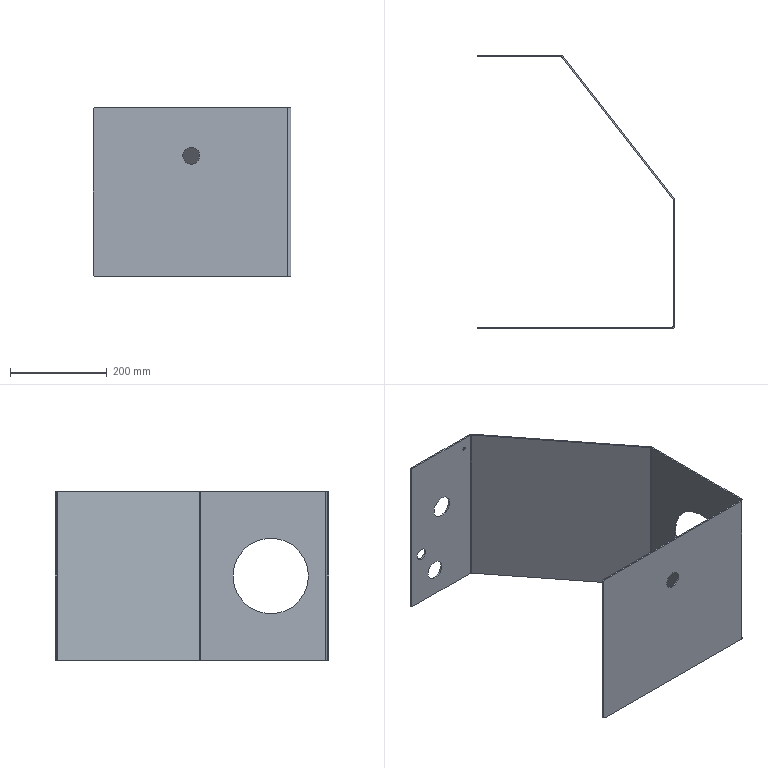Part | SolidWorks | features ICE 4, FlatPattern 1, SMBaseFlange 1, SheetMetal 1 | 1 solid | 46 faces | box 409 x 566 x 350 mm | volume 1214329 mm3 | plane 24 | cylinder 22 | commonest cylinder face diameters 10 x4 6 x3 12 x3 6.1 x2 24.2 x2 35 x2
STEP:
#1=CARTESIAN_POINT('',(152.,563.,321.95));
#2=VERTEX_POINT('',#1);
#3=CARTESIAN_POINT('',(152.,563.,328.05));
#4=VERTEX_POINT('',#3);
#5=CARTESIAN_POINT('',(152.,563.,325.));
#6=DIRECTION('',(0.,1.,0.));
#7=DIRECTION('',(0.,0.,1.));
#8=AXIS2_PLACEMENT_3D('',#5,#6,#7);
#9=CIRCLE('',#8,3.05);
#10=EDGE_CURVE('',#2,#4,#9,.T.);
#11=ORIENTED_EDGE('',*,*,#10,.F.);
#12=CARTESIAN_POINT('',(152.,566.,321.95));
#13=VERTEX_POINT('',#12);
#14=CARTESIAN_POINT('',(152.,556.,321.95));
#15=DIRECTION('',(0.,1.,0.));
#16=VECTOR('',#15,1000.);
#17=LINE('',#14,#16);
#18=EDGE_CURVE('',#2,#13,#17,.T.);
#19=ORIENTED_EDGE('',*,*,#18,.T.);
#20=CARTESIAN_POINT('',(152.,566.,328.05));
#21=VERTEX_POINT('',#20);
#22=CARTESIAN_POINT('',(152.,566.,325.));
#23=DIRECTION('',(0.,1.,0.));
#24=DIRECTION('',(0.,0.,1.));
#25=AXIS2_PLACEMENT_3D('',#22,#23,#24);
#26=CIRCLE('',#25,3.05);
#27=EDGE_CURVE('',#13,#21,#26,.T.);
#28=ORIENTED_EDGE('',*,*,#27,.T.);
#29=CARTESIAN_POINT('',(152.,556.,328.05));
#30=DIRECTION('',(0.,1.,0.));
#31=VECTOR('',#30,1000.);
#32=LINE('',#29,#31);
#33=EDGE_CURVE('',#4,#21,#32,.T.);
#34=ORIENTED_EDGE('',*,*,#33,.F.);
#35=EDGE_LOOP('',(#11,#19,#28,#34));
#36=FACE_OUTER_BOUND('',#35,.T.);
#37=CARTESIAN_POINT('',(152.,556.,325.));
#38=DIRECTION('',(0.,1.,0.));
#39=DIRECTION('',(0.,0.,1.));
#40=AXIS2_PLACEMENT_3D('',#37,#38,#39);
#41=CYLINDRICAL_SURFACE('',#40,3.05);
#42=ADVANCED_FACE('',(#36),#41,.F.);
#43=CARTESIAN_POINT('',(87.,563.,187.4));
#44=VERTEX_POINT('',#43);
#45=CARTESIAN_POINT('',(87.,563.,232.6));
#46=VERTEX_POINT('',#45);
#47=CARTESIAN_POINT('',(87.,563.,210.));
#48=DIRECTION('',(0.,1.,0.));
#49=DIRECTION('',(0.,0.,1.));
#50=AXIS2_PLACEMENT_3D('',#47,#48,#49);
#51=CIRCLE('',#50,22.6);
#52=EDGE_CURVE('',#44,#46,#51,.T.);
#53=ORIENTED_EDGE('',*,*,#52,.F.);
#54=CARTESIAN_POINT('',(87.,566.,187.4));
#55=VERTEX_POINT('',#54);
#56=CARTESIAN_POINT('',(87.,556.,187.4));
#57=DIRECTION('',(0.,1.,0.));
#58=VECTOR('',#57,1000.);
#59=LINE('',#56,#58);
#60=EDGE_CURVE('',#44,#55,#59,.T.);
#61=ORIENTED_EDGE('',*,*,#60,.T.);
#62=CARTESIAN_POINT('',(87.,566.,232.6));
#63=VERTEX_POINT('',#62);
#64=CARTESIAN_POINT('',(87.,566.,210.));
#65=DIRECTION('',(0.,1.,0.));
#66=DIRECTION('',(0.,0.,1.));
#67=AXIS2_PLACEMENT_3D('',#64,#65,#66);
#68=CIRCLE('',#67,22.6);
#69=EDGE_CURVE('',#55,#63,#68,.T.);
#70=ORIENTED_EDGE('',*,*,#69,.T.);
#71=CARTESIAN_POINT('',(87.,556.,232.6));
#72=DIRECTION('',(0.,1.,0.));
#73=VECTOR('',#72,1000.);
#74=LINE('',#71,#73);
#75=EDGE_CURVE('',#46,#63,#74,.T.);
#76=ORIENTED_EDGE('',*,*,#75,.F.);
#77=EDGE_LOOP('',(#53,#61,#70,#76));
#78=FACE_OUTER_BOUND('',#77,.T.);
#79=CARTESIAN_POINT('',(87.,556.,210.));
#80=DIRECTION('',(0.,1.,0.));
#81=DIRECTION('',(0.,0.,1.));
#82=AXIS2_PLACEMENT_3D('',#79,#80,#81);
#83=CYLINDRICAL_SURFACE('',#82,22.6);
#84=ADVANCED_FACE('',(#78),#83,.F.);
#85=CARTESIAN_POINT('',(27.,563.,107.9));
#86=VERTEX_POINT('',#85);
#87=CARTESIAN_POINT('',(27.,563.,132.1));
#88=VERTEX_POINT('',#87);
#89=CARTESIAN_POINT('',(27.,563.,120.));
#90=DIRECTION('',(0.,1.,0.));
#91=DIRECTION('',(0.,0.,1.));
#92=AXIS2_PLACEMENT_3D('',#89,#90,#91);
#93=CIRCLE('',#92,12.1);
#94=EDGE_CURVE('',#86,#88,#93,.T.);
#95=ORIENTED_EDGE('',*,*,#94,.F.);
#96=CARTESIAN_POINT('',(27.,566.,107.9));
#97=VERTEX_POINT('',#96);
#98=CARTESIAN_POINT('',(27.,556.,107.9));
#99=DIRECTION('',(0.,1.,0.));
#100=VECTOR('',#99,1000.);
#101=LINE('',#98,#100);
#102=EDGE_CURVE('',#86,#97,#101,.T.);
#103=ORIENTED_EDGE('',*,*,#102,.T.);
#104=CARTESIAN_POINT('',(27.,566.,132.1));
#105=VERTEX_POINT('',#104);
#106=CARTESIAN_POINT('',(27.,566.,120.));
#107=DIRECTION('',(0.,1.,0.));
#108=DIRECTION('',(0.,0.,1.));
#109=AXIS2_PLACEMENT_3D('',#106,#107,#108);
#110=CIRCLE('',#109,12.1);
#111=EDGE_CURVE('',#97,#105,#110,.T.);
#112=ORIENTED_EDGE('',*,*,#111,.T.);
#113=CARTESIAN_POINT('',(27.,556.,132.1));
#114=DIRECTION('',(0.,1.,0.));
#115=VECTOR('',#114,1000.);
#116=LINE('',#113,#115);
#117=EDGE_CURVE('',#88,#105,#116,.T.);
#118=ORIENTED_EDGE('',*,*,#117,.F.);
#119=EDGE_LOOP('',(#95,#103,#112,#118));
#120=FACE_OUTER_BOUND('',#119,.T.);
#121=CARTESIAN_POINT('',(27.,556.,120.));
#122=DIRECTION('',(0.,1.,0.));
#123=DIRECTION('',(0.,0.,1.));
#124=AXIS2_PLACEMENT_3D('',#121,#122,#123);
#125=CYLINDRICAL_SURFACE('',#124,12.1);
#126=ADVANCED_FACE('',(#120),#125,.F.);
#127=CARTESIAN_POINT('',(67.,563.,40.));
#128=VERTEX_POINT('',#127);
#129=CARTESIAN_POINT('',(67.,563.,80.));
#130=VERTEX_POINT('',#129);
#131=CARTESIAN_POINT('',(67.,563.,60.));
#132=DIRECTION('',(0.,1.,0.));
#133=DIRECTION('',(0.,0.,1.));
#134=AXIS2_PLACEMENT_3D('',#131,#132,#133);
#135=CIRCLE('',#134,20.);
#136=EDGE_CURVE('',#128,#130,#135,.T.);
#137=ORIENTED_EDGE('',*,*,#136,.F.);
#138=CARTESIAN_POINT('',(67.,566.,40.));
#139=VERTEX_POINT('',#138);
#140=CARTESIAN_POINT('',(67.,556.,40.));
#141=DIRECTION('',(0.,1.,0.));
#142=VECTOR('',#141,1000.);
#143=LINE('',#140,#142);
#144=EDGE_CURVE('',#128,#139,#143,.T.);
#145=ORIENTED_EDGE('',*,*,#144,.T.);
#146=CARTESIAN_POINT('',(67.,566.,80.));
#147=VERTEX_POINT('',#146);
#148=CARTESIAN_POINT('',(67.,566.,60.));
#149=DIRECTION('',(0.,1.,0.));
#150=DIRECTION('',(0.,0.,1.));
#151=AXIS2_PLACEMENT_3D('',#148,#149,#150);
#152=CIRCLE('',#151,20.);
#153=EDGE_CURVE('',#139,#147,#152,.T.);
#154=ORIENTED_EDGE('',*,*,#153,.T.);
#155=CARTESIAN_POINT('',(67.,556.,80.));
#156=DIRECTION('',(0.,1.,0.));
#157=VECTOR('',#156,1000.);
#158=LINE('',#155,#157);
#159=EDGE_CURVE('',#130,#147,#158,.T.);
#160=ORIENTED_EDGE('',*,*,#159,.F.);
#161=EDGE_LOOP('',(#137,#145,#154,#160));
#162=FACE_OUTER_BOUND('',#161,.T.);
#163=CARTESIAN_POINT('',(67.,556.,60.));
#164=DIRECTION('',(0.,1.,0.));
#165=DIRECTION('',(0.,0.,1.));
#166=AXIS2_PLACEMENT_3D('',#163,#164,#165);
#167=CYLINDRICAL_SURFACE('',#166,20.);
#168=ADVANCED_FACE('',(#162),#167,.F.);
#169=CARTESIAN_POINT('',(200.,3.,267.5));
#170=VERTEX_POINT('',#169);
#171=CARTESIAN_POINT('',(200.,3.,232.5));
#172=VERTEX_POINT('',#171);
#173=CARTESIAN_POINT('',(200.,3.,250.));
#174=DIRECTION('',(0.,-1.,0.));
#175=DIRECTION('',(0.,0.,-1.));
#176=AXIS2_PLACEMENT_3D('',#173,#174,#175);
#177=CIRCLE('',#176,17.5);
#178=EDGE_CURVE('',#170,#172,#177,.T.);
#179=ORIENTED_EDGE('',*,*,#178,.F.);
#180=CARTESIAN_POINT('',(200.,0.,267.5));
#181=VERTEX_POINT('',#180);
#182=CARTESIAN_POINT('',(200.,10.,267.5));
#183=DIRECTION('',(0.,-1.,0.));
#184=VECTOR('',#183,1000.);
#185=LINE('',#182,#184);
#186=EDGE_CURVE('',#170,#181,#185,.T.);
#187=ORIENTED_EDGE('',*,*,#186,.T.);
#188=CARTESIAN_POINT('',(200.,0.,232.5));
#189=VERTEX_POINT('',#188);
#190=CARTESIAN_POINT('',(200.,0.,250.));
#191=DIRECTION('',(0.,-1.,0.));
#192=DIRECTION('',(0.,0.,-1.));
#193=AXIS2_PLACEMENT_3D('',#190,#191,#192);
#194=CIRCLE('',#193,17.5);
#195=EDGE_CURVE('',#181,#189,#194,.T.);
#196=ORIENTED_EDGE('',*,*,#195,.T.);
#197=CARTESIAN_POINT('',(200.,10.,232.5));
#198=DIRECTION('',(0.,-1.,0.));
#199=VECTOR('',#198,1000.);
#200=LINE('',#197,#199);
#201=EDGE_CURVE('',#172,#189,#200,.T.);
#202=ORIENTED_EDGE('',*,*,#201,.F.);
#203=EDGE_LOOP('',(#179,#187,#196,#202));
#204=FACE_OUTER_BOUND('',#203,.T.);
#205=CARTESIAN_POINT('',(200.,10.,250.));
#206=DIRECTION('',(0.,-1.,0.));
#207=DIRECTION('',(0.,0.,-1.));
#208=AXIS2_PLACEMENT_3D('',#205,#206,#207);
#209=CYLINDRICAL_SURFACE('',#208,17.5);
#210=ADVANCED_FACE('',(#204),#209,.F.);
#211=CARTESIAN_POINT('',(403.,42.,175.));
#212=VERTEX_POINT('',#211);
#213=CARTESIAN_POINT('',(403.,198.,175.));
#214=VERTEX_POINT('',#213);
#215=CARTESIAN_POINT('',(403.,120.,175.));
#216=DIRECTION('',(1.,0.,0.));
#217=DIRECTION('',(0.,1.,0.));
#218=AXIS2_PLACEMENT_3D('',#215,#216,#217);
#219=CIRCLE('',#218,78.);
#220=EDGE_CURVE('',#212,#214,#219,.T.);
#221=ORIENTED_EDGE('',*,*,#220,.F.);
#222=CARTESIAN_POINT('',(406.,42.,175.));
#223=VERTEX_POINT('',#222);
#224=CARTESIAN_POINT('',(396.,42.,175.));
#225=DIRECTION('',(1.,0.,0.));
#226=VECTOR('',#225,1000.);
#227=LINE('',#224,#226);
#228=EDGE_CURVE('',#212,#223,#227,.T.);
#229=ORIENTED_EDGE('',*,*,#228,.T.);
#230=CARTESIAN_POINT('',(406.,198.,175.));
#231=VERTEX_POINT('',#230);
#232=CARTESIAN_POINT('',(406.,120.,175.));
#233=DIRECTION('',(1.,0.,0.));
#234=DIRECTION('',(0.,1.,0.));
#235=AXIS2_PLACEMENT_3D('',#232,#233,#234);
#236=CIRCLE('',#235,78.);
#237=EDGE_CURVE('',#223,#231,#236,.T.);
#238=ORIENTED_EDGE('',*,*,#237,.T.);
#239=CARTESIAN_POINT('',(396.,198.,175.));
#240=DIRECTION('',(1.,0.,0.));
#241=VECTOR('',#240,1000.);
#242=LINE('',#239,#241);
#243=EDGE_CURVE('',#214,#231,#242,.T.);
#244=ORIENTED_EDGE('',*,*,#243,.F.);
#245=EDGE_LOOP('',(#221,#229,#238,#244));
#246=FACE_OUTER_BOUND('',#245,.T.);
#247=CARTESIAN_POINT('',(396.,120.,175.));
#248=DIRECTION('',(1.,0.,0.));
#249=DIRECTION('',(0.,1.,0.));
#250=AXIS2_PLACEMENT_3D('',#247,#248,#249);
#251=CYLINDRICAL_SURFACE('',#250,78.);
#252=ADVANCED_FACE('',(#246),#251,.F.);
#253=CARTESIAN_POINT('',(152.,566.,325.));
#254=DIRECTION('',(0.,1.,0.));
#255=DIRECTION('',(0.,0.,1.));
#256=AXIS2_PLACEMENT_3D('',#253,#254,#255);
#257=CIRCLE('',#256,3.05);
#258=EDGE_CURVE('',#21,#13,#257,.T.);
#259=ORIENTED_EDGE('',*,*,#258,.F.);
#260=ORIENTED_EDGE('',*,*,#27,.F.);
#261=EDGE_LOOP('',(#259,#260));
#262=FACE_BOUND('',#261,.T.);
#263=CARTESIAN_POINT('',(87.,566.,210.));
#264=DIRECTION('',(0.,1.,0.));
#265=DIRECTION('',(0.,0.,1.));
#266=AXIS2_PLACEMENT_3D('',#263,#264,#265);
#267=CIRCLE('',#266,22.6);
#268=EDGE_CURVE('',#63,#55,#267,.T.);
#269=ORIENTED_EDGE('',*,*,#268,.F.);
#270=ORIENTED_EDGE('',*,*,#69,.F.);
#271=EDGE_LOOP('',(#269,#270));
#272=FACE_BOUND('',#271,.T.);
#273=CARTESIAN_POINT('',(27.,566.,120.));
#274=DIRECTION('',(0.,1.,0.));
#275=DIRECTION('',(0.,0.,1.));
#276=AXIS2_PLACEMENT_3D('',#273,#274,#275);
#277=CIRCLE('',#276,12.1);
#278=EDGE_CURVE('',#105,#97,#277,.T.);
#279=ORIENTED_EDGE('',*,*,#278,.F.);
#280=ORIENTED_EDGE('',*,*,#111,.F.);
#281=EDGE_LOOP('',(#279,#280));
#282=FACE_BOUND('',#281,.T.);
#283=CARTESIAN_POINT('',(67.,566.,60.));
#284=DIRECTION('',(0.,1.,0.));
#285=DIRECTION('',(0.,0.,1.));
#286=AXIS2_PLACEMENT_3D('',#283,#284,#285);
#287=CIRCLE('',#286,20.);
#288=EDGE_CURVE('',#147,#139,#287,.T.);
#289=ORIENTED_EDGE('',*,*,#288,.F.);
#290=ORIENTED_EDGE('',*,*,#153,.F.);
#291=EDGE_LOOP('',(#289,#290));
#292=FACE_BOUND('',#291,.T.);
#293=CARTESIAN_POINT('',(2.,566.,0.));
#294=VERTEX_POINT('',#293);
#295=CARTESIAN_POINT('',(170.25,566.,0.));
#296=VERTEX_POINT('',#295);
#297=CARTESIAN_POINT('',(-3.,566.,0.));
#298=DIRECTION('',(1.,0.,0.));
#299=VECTOR('',#298,1000.);
#300=LINE('',#297,#299);
#301=EDGE_CURVE('',#294,#296,#300,.T.);
#302=ORIENTED_EDGE('',*,*,#301,.F.);
#303=CARTESIAN_POINT('',(-3.,566.,5.));
#304=VERTEX_POINT('',#303);
#305=CARTESIAN_POINT('',(2.,566.,5.));
#306=DIRECTION('',(0.,-1.,0.));
#307=DIRECTION('',(0.,0.,1.));
#308=AXIS2_PLACEMENT_3D('',#305,#306,#307);
#309=CIRCLE('',#308,5.);
#310=EDGE_CURVE('',#304,#294,#309,.T.);
#311=ORIENTED_EDGE('',*,*,#310,.F.);
#312=CARTESIAN_POINT('',(-3.,566.,345.));
#313=VERTEX_POINT('',#312);
#314=CARTESIAN_POINT('',(-3.,566.,350.));
#315=DIRECTION('',(0.,0.,-1.));
#316=VECTOR('',#315,1000.);
#317=LINE('',#314,#316);
#318=EDGE_CURVE('',#313,#304,#317,.T.);
#319=ORIENTED_EDGE('',*,*,#318,.F.);
#320=CARTESIAN_POINT('',(2.,566.,350.));
#321=VERTEX_POINT('',#320);
#322=CARTESIAN_POINT('',(2.,566.,345.));
#323=DIRECTION('',(0.,-1.,0.));
#324=DIRECTION('',(0.,0.,1.));
#325=AXIS2_PLACEMENT_3D('',#322,#323,#324);
#326=CIRCLE('',#325,5.);
#327=EDGE_CURVE('',#321,#313,#326,.T.);
#328=ORIENTED_EDGE('',*,*,#327,.F.);
#329=CARTESIAN_POINT('',(170.25,566.,350.));
#330=VERTEX_POINT('',#329);
#331=CARTESIAN_POINT('',(-3.,566.,350.));
#332=DIRECTION('',(1.,0.,0.));
#333=VECTOR('',#332,1000.);
#334=LINE('',#331,#333);
#335=EDGE_CURVE('',#321,#330,#334,.T.);
#336=ORIENTED_EDGE('',*,*,#335,.T.);
#337=CARTESIAN_POINT('',(170.25,566.,350.));
#338=DIRECTION('',(0.,0.,-1.));
#339=VECTOR('',#338,1000.);
#340=LINE('',#337,#339);
#341=EDGE_CURVE('',#330,#296,#340,.T.);
#342=ORIENTED_EDGE('',*,*,#341,.T.);
#343=EDGE_LOOP('',(#302,#311,#319,#328,#336,#342));
#344=FACE_OUTER_BOUND('',#343,.T.);
#345=CARTESIAN_POINT('',(-3.,566.,350.));
#346=DIRECTION('',(0.,1.,0.));
#347=DIRECTION('',(0.,0.,1.));
#348=AXIS2_PLACEMENT_3D('',#345,#346,#347);
#349=PLANE('',#348);
#350=ADVANCED_FACE('',(#262,#272,#282,#292,#344),#349,.T.);
#351=CARTESIAN_POINT('',(152.,563.,325.));
#352=DIRECTION('',(0.,1.,0.));
#353=DIRECTION('',(0.,0.,1.));
#354=AXIS2_PLACEMENT_3D('',#351,#352,#353);
#355=CIRCLE('',#354,3.05);
#356=EDGE_CURVE('',#4,#2,#355,.T.);
#357=ORIENTED_EDGE('',*,*,#356,.T.);
#358=ORIENTED_EDGE('',*,*,#10,.T.);
#359=EDGE_LOOP('',(#357,#358));
#360=FACE_BOUND('',#359,.T.);
#361=CARTESIAN_POINT('',(87.,563.,210.));
#362=DIRECTION('',(0.,1.,0.));
#363=DIRECTION('',(0.,0.,1.));
#364=AXIS2_PLACEMENT_3D('',#361,#362,#363);
#365=CIRCLE('',#364,22.6);
#366=EDGE_CURVE('',#46,#44,#365,.T.);
#367=ORIENTED_EDGE('',*,*,#366,.T.);
#368=ORIENTED_EDGE('',*,*,#52,.T.);
#369=EDGE_LOOP('',(#367,#368));
#370=FACE_BOUND('',#369,.T.);
#371=CARTESIAN_POINT('',(27.,563.,120.));
#372=DIRECTION('',(0.,1.,0.));
#373=DIRECTION('',(0.,0.,1.));
#374=AXIS2_PLACEMENT_3D('',#371,#372,#373);
#375=CIRCLE('',#374,12.1);
#376=EDGE_CURVE('',#88,#86,#375,.T.);
#377=ORIENTED_EDGE('',*,*,#376,.T.);
#378=ORIENTED_EDGE('',*,*,#94,.T.);
#379=EDGE_LOOP('',(#377,#378));
#380=FACE_BOUND('',#379,.T.);
#381=CARTESIAN_POINT('',(67.,563.,60.));
#382=DIRECTION('',(0.,1.,0.));
#383=DIRECTION('',(0.,0.,1.));
#384=AXIS2_PLACEMENT_3D('',#381,#382,#383);
#385=CIRCLE('',#384,20.);
#386=EDGE_CURVE('',#130,#128,#385,.T.);
#387=ORIENTED_EDGE('',*,*,#386,.T.);
#388=ORIENTED_EDGE('',*,*,#136,.T.);
#389=EDGE_LOOP('',(#387,#388));
#390=FACE_BOUND('',#389,.T.);
#391=CARTESIAN_POINT('',(-3.,563.,5.));
#392=VERTEX_POINT('',#391);
#393=CARTESIAN_POINT('',(2.,563.,0.));
#394=VERTEX_POINT('',#393);
#395=CARTESIAN_POINT('',(2.,563.,5.));
#396=DIRECTION('',(0.,-1.,0.));
#397=DIRECTION('',(0.,0.,1.));
#398=AXIS2_PLACEMENT_3D('',#395,#396,#397);
#399=CIRCLE('',#398,5.);
#400=EDGE_CURVE('',#392,#394,#399,.T.);
#401=ORIENTED_EDGE('',*,*,#400,.T.);
#402=CARTESIAN_POINT('',(170.25,563.,0.));
#403=VERTEX_POINT('',#402);
#404=CARTESIAN_POINT('',(-3.,563.,0.));
#405=DIRECTION('',(1.,0.,0.));
#406=VECTOR('',#405,1000.);
#407=LINE('',#404,#406);
#408=EDGE_CURVE('',#394,#403,#407,.T.);
#409=ORIENTED_EDGE('',*,*,#408,.T.);
#410=CARTESIAN_POINT('',(170.25,563.,350.));
#411=VERTEX_POINT('',#410);
#412=CARTESIAN_POINT('',(170.25,563.,350.));
#413=DIRECTION('',(0.,0.,-1.));
#414=VECTOR('',#413,1000.);
#415=LINE('',#412,#414);
#416=EDGE_CURVE('',#411,#403,#415,.T.);
#417=ORIENTED_EDGE('',*,*,#416,.F.);
#418=CARTESIAN_POINT('',(2.,563.,350.));
#419=VERTEX_POINT('',#418);
#420=CARTESIAN_POINT('',(-3.,563.,350.));
#421=DIRECTION('',(1.,0.,0.));
#422=VECTOR('',#421,1000.);
#423=LINE('',#420,#422);
#424=EDGE_CURVE('',#419,#411,#423,.T.);
#425=ORIENTED_EDGE('',*,*,#424,.F.);
#426=CARTESIAN_POINT('',(-3.,563.,345.));
#427=VERTEX_POINT('',#426);
#428=CARTESIAN_POINT('',(2.,563.,345.));
#429=DIRECTION('',(0.,-1.,0.));
#430=DIRECTION('',(0.,0.,1.));
#431=AXIS2_PLACEMENT_3D('',#428,#429,#430);
#432=CIRCLE('',#431,5.);
#433=EDGE_CURVE('',#419,#427,#432,.T.);
#434=ORIENTED_EDGE('',*,*,#433,.T.);
#435=CARTESIAN_POINT('',(-3.,563.,350.));
#436=DIRECTION('',(0.,0.,-1.));
#437=VECTOR('',#436,1000.);
#438=LINE('',#435,#437);
#439=EDGE_CURVE('',#427,#392,#438,.T.);
#440=ORIENTED_EDGE('',*,*,#439,.T.);
#441=EDGE_LOOP('',(#401,#409,#417,#425,#434,#440));
#442=FACE_OUTER_BOUND('',#441,.T.);
#443=CARTESIAN_POINT('',(-3.,563.,350.));
#444=DIRECTION('',(0.,1.,0.));
#445=DIRECTION('',(0.,0.,1.));
#446=AXIS2_PLACEMENT_3D('',#443,#444,#445);
#447=PLANE('',#446);
#448=ADVANCED_FACE('',(#360,#370,#380,#390,#442),#447,.F.);
#449=ORIENTED_EDGE('',*,*,#408,.F.);
#450=CARTESIAN_POINT('',(2.,563.,0.));
#451=DIRECTION('',(0.,1.,0.));
#452=VECTOR('',#451,1000.);
#453=LINE('',#450,#452);
#454=EDGE_CURVE('',#394,#294,#453,.T.);
#455=ORIENTED_EDGE('',*,*,#454,.T.);
#456=ORIENTED_EDGE('',*,*,#301,.T.);
#457=CARTESIAN_POINT('',(170.25,566.,0.));
#458=DIRECTION('',(0.,-1.,0.));
#459=VECTOR('',#458,1000.);
#460=LINE('',#457,#459);
#461=EDGE_CURVE('',#296,#403,#460,.T.);
#462=ORIENTED_EDGE('',*,*,#461,.T.);
#463=EDGE_LOOP('',(#449,#455,#456,#462));
#464=FACE_OUTER_BOUND('',#463,.T.);
#465=CARTESIAN_POINT('',(172.615,561.847,0.));
#466=DIRECTION('',(0.,0.,-1.));
#467=DIRECTION('',(-1.,0.,0.));
#468=AXIS2_PLACEMENT_3D('',#465,#466,#467);
#469=PLANE('',#468);
#470=ADVANCED_FACE('',(#464),#469,.T.);
#471=CARTESIAN_POINT('',(200.,0.,250.));
#472=DIRECTION('',(0.,-1.,0.));
#473=DIRECTION('',(0.,0.,-1.));
#474=AXIS2_PLACEMENT_3D('',#471,#472,#473);
#475=CIRCLE('',#474,17.5);
#476=EDGE_CURVE('',#189,#181,#475,.T.);
#477=ORIENTED_EDGE('',*,*,#476,.F.);
#478=ORIENTED_EDGE('',*,*,#195,.F.);
#479=EDGE_LOOP('',(#477,#478));
#480=FACE_BOUND('',#479,.T.);
#481=CARTESIAN_POINT('',(-3.,0.,345.));
#482=VERTEX_POINT('',#481);
#483=CARTESIAN_POINT('',(-3.,0.,5.));
#484=VERTEX_POINT('',#483);
#485=CARTESIAN_POINT('',(-3.,0.,350.));
#486=DIRECTION('',(0.,0.,-1.));
#487=VECTOR('',#486,1000.);
#488=LINE('',#485,#487);
#489=EDGE_CURVE('',#482,#484,#488,.T.);
#490=ORIENTED_EDGE('',*,*,#489,.T.);
#491=CARTESIAN_POINT('',(2.,0.,0.));
#492=VERTEX_POINT('',#491);
#493=CARTESIAN_POINT('',(2.,0.,5.));
#494=DIRECTION('',(0.,1.,0.));
#495=DIRECTION('',(0.,0.,-1.));
#496=AXIS2_PLACEMENT_3D('',#493,#494,#495);
#497=CIRCLE('',#496,5.);
#498=EDGE_CURVE('',#492,#484,#497,.T.);
#499=ORIENTED_EDGE('',*,*,#498,.F.);
#500=CARTESIAN_POINT('',(400.,0.,0.));
#501=VERTEX_POINT('',#500);
#502=CARTESIAN_POINT('',(0.,0.,0.));
#503=DIRECTION('',(-1.,0.,0.));
#504=VECTOR('',#503,1000.);
#505=LINE('',#502,#504);
#506=EDGE_CURVE('',#501,#492,#505,.T.);
#507=ORIENTED_EDGE('',*,*,#506,.F.);
#508=CARTESIAN_POINT('',(400.,0.,350.));
#509=VERTEX_POINT('',#508);
#510=CARTESIAN_POINT('',(400.,0.,350.));
#511=DIRECTION('',(0.,0.,-1.));
#512=VECTOR('',#511,1000.);
#513=LINE('',#510,#512);
#514=EDGE_CURVE('',#509,#501,#513,.T.);
#515=ORIENTED_EDGE('',*,*,#514,.F.);
#516=CARTESIAN_POINT('',(2.,0.,350.));
#517=VERTEX_POINT('',#516);
#518=CARTESIAN_POINT('',(0.,0.,350.));
#519=DIRECTION('',(-1.,0.,0.));
#520=VECTOR('',#519,1000.);
#521=LINE('',#518,#520);
#522=EDGE_CURVE('',#509,#517,#521,.T.);
#523=ORIENTED_EDGE('',*,*,#522,.T.);
#524=CARTESIAN_POINT('',(2.,0.,345.));
#525=DIRECTION('',(0.,1.,0.));
#526=DIRECTION('',(0.,0.,-1.));
#527=AXIS2_PLACEMENT_3D('',#524,#525,#526);
#528=CIRCLE('',#527,5.);
#529=EDGE_CURVE('',#482,#517,#528,.T.);
#530=ORIENTED_EDGE('',*,*,#529,.F.);
#531=EDGE_LOOP('',(#490,#499,#507,#515,#523,#530));
#532=FACE_OUTER_BOUND('',#531,.T.);
#533=CARTESIAN_POINT('',(0.,0.,350.));
#534=DIRECTION('',(0.,-1.,0.));
#535=DIRECTION('',(0.,0.,-1.));
#536=AXIS2_PLACEMENT_3D('',#533,#534,#535);
#537=PLANE('',#536);
#538=ADVANCED_FACE('',(#480,#532),#537,.T.);
#539=CARTESIAN_POINT('',(200.,3.,250.));
#540=DIRECTION('',(0.,-1.,0.));
#541=DIRECTION('',(0.,0.,-1.));
#542=AXIS2_PLACEMENT_3D('',#539,#540,#541);
#543=CIRCLE('',#542,17.5);
#544=EDGE_CURVE('',#172,#170,#543,.T.);
#545=ORIENTED_EDGE('',*,*,#544,.T.);
#546=ORIENTED_EDGE('',*,*,#178,.T.);
#547=EDGE_LOOP('',(#545,#546));
#548=FACE_BOUND('',#547,.T.);
#549=CARTESIAN_POINT('',(2.,3.,0.));
#550=VERTEX_POINT('',#549);
#551=CARTESIAN_POINT('',(-3.,3.,5.));
#552=VERTEX_POINT('',#551);
#553=CARTESIAN_POINT('',(2.,3.,5.));
#554=DIRECTION('',(0.,1.,0.));
#555=DIRECTION('',(0.,0.,-1.));
#556=AXIS2_PLACEMENT_3D('',#553,#554,#555);
#557=CIRCLE('',#556,5.);
#558=EDGE_CURVE('',#550,#552,#557,.T.);
#559=ORIENTED_EDGE('',*,*,#558,.T.);
#560=CARTESIAN_POINT('',(-3.,3.,345.));
#561=VERTEX_POINT('',#560);
#562=CARTESIAN_POINT('',(-3.,3.,350.));
#563=DIRECTION('',(0.,0.,-1.));
#564=VECTOR('',#563,1000.);
#565=LINE('',#562,#564);
#566=EDGE_CURVE('',#561,#552,#565,.T.);
#567=ORIENTED_EDGE('',*,*,#566,.F.);
#568=CARTESIAN_POINT('',(2.,3.,350.));
#569=VERTEX_POINT('',#568);
#570=CARTESIAN_POINT('',(2.,3.,345.));
#571=DIRECTION('',(0.,1.,0.));
#572=DIRECTION('',(0.,0.,-1.));
#573=AXIS2_PLACEMENT_3D('',#570,#571,#572);
#574=CIRCLE('',#573,5.);
#575=EDGE_CURVE('',#561,#569,#574,.T.);
#576=ORIENTED_EDGE('',*,*,#575,.T.);
#577=CARTESIAN_POINT('',(400.,3.,350.));
#578=VERTEX_POINT('',#577);
#579=CARTESIAN_POINT('',(0.,3.,350.));
#580=DIRECTION('',(-1.,0.,0.));
#581=VECTOR('',#580,1000.);
#582=LINE('',#579,#581);
#583=EDGE_CURVE('',#578,#569,#582,.T.);
#584=ORIENTED_EDGE('',*,*,#583,.F.);
#585=CARTESIAN_POINT('',(400.,3.,0.));
#586=VERTEX_POINT('',#585);
#587=CARTESIAN_POINT('',(400.,3.,350.));
#588=DIRECTION('',(0.,0.,-1.));
#589=VECTOR('',#588,1000.);
#590=LINE('',#587,#589);
#591=EDGE_CURVE('',#578,#586,#590,.T.);
#592=ORIENTED_EDGE('',*,*,#591,.T.);
#593=CARTESIAN_POINT('',(0.,3.,0.));
#594=DIRECTION('',(-1.,0.,0.));
#595=VECTOR('',#594,1000.);
#596=LINE('',#593,#595);
#597=EDGE_CURVE('',#586,#550,#596,.T.);
#598=ORIENTED_EDGE('',*,*,#597,.T.);
#599=EDGE_LOOP('',(#559,#567,#576,#584,#592,#598));
#600=FACE_OUTER_BOUND('',#599,.T.);
#601=CARTESIAN_POINT('',(0.,3.,350.));
#602=DIRECTION('',(0.,-1.,0.));
#603=DIRECTION('',(0.,0.,-1.));
#604=AXIS2_PLACEMENT_3D('',#601,#602,#603);
#605=PLANE('',#604);
#606=ADVANCED_FACE('',(#548,#600),#605,.F.);
#607=ORIENTED_EDGE('',*,*,#566,.T.);
#608=CARTESIAN_POINT('',(-3.,3.,5.));
#609=DIRECTION('',(0.,-1.,0.));
#610=VECTOR('',#609,1000.);
#611=LINE('',#608,#610);
#612=EDGE_CURVE('',#552,#484,#611,.T.);
#613=ORIENTED_EDGE('',*,*,#612,.T.);
#614=ORIENTED_EDGE('',*,*,#489,.F.);
#615=CARTESIAN_POINT('',(-3.,3.,345.));
#616=DIRECTION('',(0.,-1.,0.));
#617=VECTOR('',#616,1000.);
#618=LINE('',#615,#617);
#619=EDGE_CURVE('',#561,#482,#618,.T.);
#620=ORIENTED_EDGE('',*,*,#619,.F.);
#621=EDGE_LOOP('',(#607,#613,#614,#620));
#622=FACE_OUTER_BOUND('',#621,.T.);
#623=CARTESIAN_POINT('',(-3.,0.,350.));
#624=DIRECTION('',(-1.,0.,0.));
#625=DIRECTION('',(0.,-1.,0.));
#626=AXIS2_PLACEMENT_3D('',#623,#624,#625);
#627=PLANE('',#626);
#628=ADVANCED_FACE('',(#622),#627,.T.);
#629=CARTESIAN_POINT('',(-3.,563.,5.));
#630=DIRECTION('',(0.,1.,0.));
#631=VECTOR('',#630,1000.);
#632=LINE('',#629,#631);
#633=EDGE_CURVE('',#392,#304,#632,.T.);
#634=ORIENTED_EDGE('',*,*,#633,.F.);
#635=ORIENTED_EDGE('',*,*,#439,.F.);
#636=CARTESIAN_POINT('',(-3.,563.,345.));
#637=DIRECTION('',(0.,1.,0.));
#638=VECTOR('',#637,1000.);
#639=LINE('',#636,#638);
#640=EDGE_CURVE('',#427,#313,#639,.T.);
#641=ORIENTED_EDGE('',*,*,#640,.T.);
#642=ORIENTED_EDGE('',*,*,#318,.T.);
#643=EDGE_LOOP('',(#634,#635,#641,#642));
#644=FACE_OUTER_BOUND('',#643,.T.);
#645=CARTESIAN_POINT('',(-3.,563.,350.));
#646=DIRECTION('',(-1.,0.,0.));
#647=DIRECTION('',(0.,0.,1.));
#648=AXIS2_PLACEMENT_3D('',#645,#646,#647);
#649=PLANE('',#648);
#650=ADVANCED_FACE('',(#644),#649,.T.);
#651=CARTESIAN_POINT('',(2.,563.,350.));
#652=DIRECTION('',(0.,1.,0.));
#653=VECTOR('',#652,1000.);
#654=LINE('',#651,#653);
#655=EDGE_CURVE('',#419,#321,#654,.T.);
#656=ORIENTED_EDGE('',*,*,#655,.F.);
#657=ORIENTED_EDGE('',*,*,#424,.T.);
#658=CARTESIAN_POINT('',(170.25,563.,350.));
#659=DIRECTION('',(0.,1.,0.));
#660=VECTOR('',#659,1000.);
#661=LINE('',#658,#660);
#662=EDGE_CURVE('',#411,#330,#661,.T.);
#663=ORIENTED_EDGE('',*,*,#662,.T.);
#664=ORIENTED_EDGE('',*,*,#335,.F.);
#665=EDGE_LOOP('',(#656,#657,#663,#664));
#666=FACE_OUTER_BOUND('',#665,.T.);
#667=CARTESIAN_POINT('',(400.,6.,350.));
#668=DIRECTION('',(0.,0.,-1.));
#669=DIRECTION('',(-1.,0.,0.));
#670=AXIS2_PLACEMENT_3D('',#667,#668,#669);
#671=PLANE('',#670);
#672=ADVANCED_FACE('',(#666),#671,.F.);
#673=ORIENTED_EDGE('',*,*,#583,.T.);
#674=CARTESIAN_POINT('',(2.,3.,350.));
#675=DIRECTION('',(0.,-1.,0.));
#676=VECTOR('',#675,1000.);
#677=LINE('',#674,#676);
#678=EDGE_CURVE('',#569,#517,#677,.T.);
#679=ORIENTED_EDGE('',*,*,#678,.T.);
#680=ORIENTED_EDGE('',*,*,#522,.F.);
#681=CARTESIAN_POINT('',(400.,0.,350.));
#682=DIRECTION('',(0.,1.,0.));
#683=VECTOR('',#682,1000.);
#684=LINE('',#681,#683);
#685=EDGE_CURVE('',#509,#578,#684,.T.);
#686=ORIENTED_EDGE('',*,*,#685,.T.);
#687=EDGE_LOOP('',(#673,#679,#680,#686));
#688=FACE_OUTER_BOUND('',#687,.T.);
#689=CARTESIAN_POINT('',(403.,6.,350.));
#690=DIRECTION('',(0.,0.,1.));
#691=DIRECTION('',(1.,0.,0.));
#692=AXIS2_PLACEMENT_3D('',#689,#690,#691);
#693=PLANE('',#692);
#694=ADVANCED_FACE('',(#688),#693,.T.);
#695=ORIENTED_EDGE('',*,*,#685,.F.);
#696=CARTESIAN_POINT('',(406.,6.,350.));
#697=VERTEX_POINT('',#696);
#698=CARTESIAN_POINT('',(400.,6.,350.));
#699=DIRECTION('',(0.,0.,-1.));
#700=DIRECTION('',(-1.,0.,0.));
#701=AXIS2_PLACEMENT_3D('',#698,#699,#700);
#702=CIRCLE('',#701,6.);
#703=EDGE_CURVE('',#697,#509,#702,.T.);
#704=ORIENTED_EDGE('',*,*,#703,.F.);
#705=CARTESIAN_POINT('',(403.,6.,350.));
#706=VERTEX_POINT('',#705);
#707=CARTESIAN_POINT('',(403.,6.,350.));
#708=DIRECTION('',(1.,0.,0.));
#709=VECTOR('',#708,1000.);
#710=LINE('',#707,#709);
#711=EDGE_CURVE('',#706,#697,#710,.T.);
#712=ORIENTED_EDGE('',*,*,#711,.F.);
#713=CARTESIAN_POINT('',(400.,6.,350.));
#714=DIRECTION('',(0.,0.,-1.));
#715=DIRECTION('',(1.,0.,0.));
#716=AXIS2_PLACEMENT_3D('',#713,#714,#715);
#717=CIRCLE('',#716,3.);
#718=EDGE_CURVE('',#706,#578,#717,.T.);
#719=ORIENTED_EDGE('',*,*,#718,.T.);
#720=EDGE_LOOP('',(#695,#704,#712,#719));
#721=FACE_OUTER_BOUND('',#720,.T.);
#722=CARTESIAN_POINT('',(400.,0.,350.));
#723=DIRECTION('',(0.,0.,1.));
#724=DIRECTION('',(1.,0.,0.));
#725=AXIS2_PLACEMENT_3D('',#722,#723,#724);
#726=PLANE('',#725);
#727=ADVANCED_FACE('',(#721),#726,.T.);
#728=CARTESIAN_POINT('',(406.,6.,0.));
#729=VERTEX_POINT('',#728);
#730=CARTESIAN_POINT('',(403.,6.,0.));
#731=VERTEX_POINT('',#730);
#732=CARTESIAN_POINT('',(406.,6.,0.));
#733=DIRECTION('',(-1.,0.,0.));
#734=VECTOR('',#733,1000.);
#735=LINE('',#732,#734);
#736=EDGE_CURVE('',#729,#731,#735,.T.);
#737=ORIENTED_EDGE('',*,*,#736,.F.);
#738=CARTESIAN_POINT('',(400.,6.,0.));
#739=DIRECTION('',(0.,0.,-1.));
#740=DIRECTION('',(-1.,0.,0.));
#741=AXIS2_PLACEMENT_3D('',#738,#739,#740);
#742=CIRCLE('',#741,6.);
#743=EDGE_CURVE('',#729,#501,#742,.T.);
#744=ORIENTED_EDGE('',*,*,#743,.T.);
#745=CARTESIAN_POINT('',(400.,3.,0.));
#746=DIRECTION('',(0.,-1.,0.));
#747=VECTOR('',#746,1000.);
#748=LINE('',#745,#747);
#749=EDGE_CURVE('',#586,#501,#748,.T.);
#750=ORIENTED_EDGE('',*,*,#749,.F.);
#751=CARTESIAN_POINT('',(400.,6.,0.));
#752=DIRECTION('',(0.,0.,-1.));
#753=DIRECTION('',(1.,0.,0.));
#754=AXIS2_PLACEMENT_3D('',#751,#752,#753);
#755=CIRCLE('',#754,3.);
#756=EDGE_CURVE('',#731,#586,#755,.T.);
#757=ORIENTED_EDGE('',*,*,#756,.F.);
#758=EDGE_LOOP('',(#737,#744,#750,#757));
#759=FACE_OUTER_BOUND('',#758,.T.);
#760=CARTESIAN_POINT('',(406.,6.,0.));
#761=DIRECTION('',(0.,0.,-1.));
#762=DIRECTION('',(-1.,0.,0.));
#763=AXIS2_PLACEMENT_3D('',#760,#761,#762);
#764=PLANE('',#763);
#765=ADVANCED_FACE('',(#759),#764,.T.);
#766=CARTESIAN_POINT('',(406.,265.934,0.));
#767=VERTEX_POINT('',#766);
#768=CARTESIAN_POINT('',(406.,0.,0.));
#769=DIRECTION('',(0.,-1.,0.));
#770=VECTOR('',#769,1000.);
#771=LINE('',#768,#770);
#772=EDGE_CURVE('',#767,#729,#771,.T.);
#773=ORIENTED_EDGE('',*,*,#772,.T.);
#774=ORIENTED_EDGE('',*,*,#736,.T.);
#775=CARTESIAN_POINT('',(403.,265.934,0.));
#776=VERTEX_POINT('',#775);
#777=CARTESIAN_POINT('',(403.,0.,0.));
#778=DIRECTION('',(0.,-1.,0.));
#779=VECTOR('',#778,1000.);
#780=LINE('',#777,#779);
#781=EDGE_CURVE('',#776,#731,#780,.T.);
#782=ORIENTED_EDGE('',*,*,#781,.F.);
#783=CARTESIAN_POINT('',(403.,265.934,0.));
#784=DIRECTION('',(1.,0.,0.));
#785=VECTOR('',#784,1000.);
#786=LINE('',#783,#785);
#787=EDGE_CURVE('',#776,#767,#786,.T.);
#788=ORIENTED_EDGE('',*,*,#787,.T.);
#789=EDGE_LOOP('',(#773,#774,#782,#788));
#790=FACE_OUTER_BOUND('',#789,.T.);
#791=CARTESIAN_POINT('',(400.,3.,0.));
#792=DIRECTION('',(0.,0.,-1.));
#793=DIRECTION('',(-1.,0.,0.));
#794=AXIS2_PLACEMENT_3D('',#791,#792,#793);
#795=PLANE('',#794);
#796=ADVANCED_FACE('',(#790),#795,.T.);
#797=CARTESIAN_POINT('',(406.,265.934,350.));
#798=VERTEX_POINT('',#797);
#799=CARTESIAN_POINT('',(403.,265.934,350.));
#800=VERTEX_POINT('',#799);
#801=CARTESIAN_POINT('',(406.,265.934,350.));
#802=DIRECTION('',(-1.,0.,0.));
#803=VECTOR('',#802,1000.);
#804=LINE('',#801,#803);
#805=EDGE_CURVE('',#798,#800,#804,.T.);
#806=ORIENTED_EDGE('',*,*,#805,.F.);
#807=CARTESIAN_POINT('',(404.728,269.628,350.));
#808=VERTEX_POINT('',#807);
#809=CARTESIAN_POINT('',(400.,265.934,350.));
#810=DIRECTION('',(0.,0.,-1.));
#811=DIRECTION('',(-1.,0.,0.));
#812=AXIS2_PLACEMENT_3D('',#809,#810,#811);
#813=CIRCLE('',#812,6.);
#814=EDGE_CURVE('',#808,#798,#813,.T.);
#815=ORIENTED_EDGE('',*,*,#814,.F.);
#816=CARTESIAN_POINT('',(402.364,267.781,350.));
#817=VERTEX_POINT('',#816);
#818=CARTESIAN_POINT('',(402.364,267.781,350.));
#819=DIRECTION('',(0.788,0.6157,0.));
#820=VECTOR('',#819,1000.);
#821=LINE('',#818,#820);
#822=EDGE_CURVE('',#817,#808,#821,.T.);
#823=ORIENTED_EDGE('',*,*,#822,.F.);
#824=CARTESIAN_POINT('',(400.,265.934,350.));
#825=DIRECTION('',(0.,0.,-1.));
#826=DIRECTION('',(1.,0.,0.));
#827=AXIS2_PLACEMENT_3D('',#824,#825,#826);
#828=CIRCLE('',#827,3.);
#829=EDGE_CURVE('',#817,#800,#828,.T.);
#830=ORIENTED_EDGE('',*,*,#829,.T.);
#831=EDGE_LOOP('',(#806,#815,#823,#830));
#832=FACE_OUTER_BOUND('',#831,.T.);
#833=CARTESIAN_POINT('',(406.,265.934,350.));
#834=DIRECTION('',(0.,0.,1.));
#835=DIRECTION('',(1.,0.,0.));
#836=AXIS2_PLACEMENT_3D('',#833,#834,#835);
#837=PLANE('',#836);
#838=ADVANCED_FACE('',(#832),#837,.T.);
#839=CARTESIAN_POINT('',(406.,0.,350.));
#840=DIRECTION('',(0.,-1.,0.));
#841=VECTOR('',#840,1000.);
#842=LINE('',#839,#841);
#843=EDGE_CURVE('',#798,#697,#842,.T.);
#844=ORIENTED_EDGE('',*,*,#843,.F.);
#845=ORIENTED_EDGE('',*,*,#805,.T.);
#846=CARTESIAN_POINT('',(403.,0.,350.));
#847=DIRECTION('',(0.,-1.,0.));
#848=VECTOR('',#847,1000.);
#849=LINE('',#846,#848);
#850=EDGE_CURVE('',#800,#706,#849,.T.);
#851=ORIENTED_EDGE('',*,*,#850,.T.);
#852=ORIENTED_EDGE('',*,*,#711,.T.);
#853=EDGE_LOOP('',(#844,#845,#851,#852));
#854=FACE_OUTER_BOUND('',#853,.T.);
#855=CARTESIAN_POINT('',(402.364,267.781,350.));
#856=DIRECTION('',(0.,0.,1.));
#857=DIRECTION('',(1.,0.,0.));
#858=AXIS2_PLACEMENT_3D('',#855,#856,#857);
#859=PLANE('',#858);
#860=ADVANCED_FACE('',(#854),#859,.T.);
#861=CARTESIAN_POINT('',(404.728,269.628,0.));
#862=VERTEX_POINT('',#861);
#863=CARTESIAN_POINT('',(402.364,267.781,0.));
#864=VERTEX_POINT('',#863);
#865=CARTESIAN_POINT('',(404.728,269.628,0.));
#866=DIRECTION('',(-0.788,-0.6157,0.));
#867=VECTOR('',#866,1000.);
#868=LINE('',#865,#867);
#869=EDGE_CURVE('',#862,#864,#868,.T.);
#870=ORIENTED_EDGE('',*,*,#869,.F.);
#871=CARTESIAN_POINT('',(400.,265.934,0.));
#872=DIRECTION('',(0.,0.,-1.));
#873=DIRECTION('',(-1.,0.,0.));
#874=AXIS2_PLACEMENT_3D('',#871,#872,#873);
#875=CIRCLE('',#874,6.);
#876=EDGE_CURVE('',#862,#767,#875,.T.);
#877=ORIENTED_EDGE('',*,*,#876,.T.);
#878=ORIENTED_EDGE('',*,*,#787,.F.);
#879=CARTESIAN_POINT('',(400.,265.934,0.));
#880=DIRECTION('',(0.,0.,-1.));
#881=DIRECTION('',(1.,0.,0.));
#882=AXIS2_PLACEMENT_3D('',#879,#880,#881);
#883=CIRCLE('',#882,3.);
#884=EDGE_CURVE('',#864,#776,#883,.T.);
#885=ORIENTED_EDGE('',*,*,#884,.F.);
#886=EDGE_LOOP('',(#870,#877,#878,#885));
#887=FACE_OUTER_BOUND('',#886,.T.);
#888=CARTESIAN_POINT('',(404.728,269.628,0.));
#889=DIRECTION('',(0.,0.,-1.));
#890=DIRECTION('',(-1.,0.,0.));
#891=AXIS2_PLACEMENT_3D('',#888,#889,#890);
#892=PLANE('',#891);
#893=ADVANCED_FACE('',(#887),#892,.T.);
#894=CARTESIAN_POINT('',(174.979,563.694,0.));
#895=VERTEX_POINT('',#894);
#896=CARTESIAN_POINT('',(406.,268.,0.));
#897=DIRECTION('',(0.6157,-0.788,0.));
#898=VECTOR('',#897,1000.);
#899=LINE('',#896,#898);
#900=EDGE_CURVE('',#895,#862,#899,.T.);
#901=ORIENTED_EDGE('',*,*,#900,.T.);
#902=ORIENTED_EDGE('',*,*,#869,.T.);
#903=CARTESIAN_POINT('',(172.615,561.847,0.));
#904=VERTEX_POINT('',#903);
#905=CARTESIAN_POINT('',(403.636,266.153,0.));
#906=DIRECTION('',(0.6157,-0.788,0.));
#907=VECTOR('',#906,1000.);
#908=LINE('',#905,#907);
#909=EDGE_CURVE('',#904,#864,#908,.T.);
#910=ORIENTED_EDGE('',*,*,#909,.F.);
#911=CARTESIAN_POINT('',(172.615,561.847,0.));
#912=DIRECTION('',(0.788,0.6157,0.));
#913=VECTOR('',#912,1000.);
#914=LINE('',#911,#913);
#915=EDGE_CURVE('',#904,#895,#914,.T.);
#916=ORIENTED_EDGE('',*,*,#915,.T.);
#917=EDGE_LOOP('',(#901,#902,#910,#916));
#918=FACE_OUTER_BOUND('',#917,.T.);
#919=CARTESIAN_POINT('',(403.,265.934,0.));
#920=DIRECTION('',(0.,0.,-1.));
#921=DIRECTION('',(-1.,0.,0.));
#922=AXIS2_PLACEMENT_3D('',#919,#920,#921);
#923=PLANE('',#922);
#924=ADVANCED_FACE('',(#918),#923,.T.);
#925=CARTESIAN_POINT('',(174.979,563.694,350.));
#926=VERTEX_POINT('',#925);
#927=CARTESIAN_POINT('',(172.615,561.847,350.));
#928=VERTEX_POINT('',#927);
#929=CARTESIAN_POINT('',(174.979,563.694,350.));
#930=DIRECTION('',(-0.788,-0.6157,0.));
#931=VECTOR('',#930,1000.);
#932=LINE('',#929,#931);
#933=EDGE_CURVE('',#926,#928,#932,.T.);
#934=ORIENTED_EDGE('',*,*,#933,.F.);
#935=CARTESIAN_POINT('',(170.25,560.,350.));
#936=DIRECTION('',(0.,0.,-1.));
#937=DIRECTION('',(-1.,0.,0.));
#938=AXIS2_PLACEMENT_3D('',#935,#936,#937);
#939=CIRCLE('',#938,6.);
#940=EDGE_CURVE('',#330,#926,#939,.T.);
#941=ORIENTED_EDGE('',*,*,#940,.F.);
#942=ORIENTED_EDGE('',*,*,#662,.F.);
#943=CARTESIAN_POINT('',(170.25,560.,350.));
#944=DIRECTION('',(0.,0.,-1.));
#945=DIRECTION('',(1.,0.,0.));
#946=AXIS2_PLACEMENT_3D('',#943,#944,#945);
#947=CIRCLE('',#946,3.);
#948=EDGE_CURVE('',#411,#928,#947,.T.);
#949=ORIENTED_EDGE('',*,*,#948,.T.);
#950=EDGE_LOOP('',(#934,#941,#942,#949));
#951=FACE_OUTER_BOUND('',#950,.T.);
#952=CARTESIAN_POINT('',(174.979,563.694,350.));
#953=DIRECTION('',(0.,0.,1.));
#954=DIRECTION('',(1.,0.,0.));
#955=AXIS2_PLACEMENT_3D('',#952,#953,#954);
#956=PLANE('',#955);
#957=ADVANCED_FACE('',(#951),#956,.T.);
#958=CARTESIAN_POINT('',(406.,268.,350.));
#959=DIRECTION('',(0.6157,-0.788,0.));
#960=VECTOR('',#959,1000.);
#961=LINE('',#958,#960);
#962=EDGE_CURVE('',#926,#808,#961,.T.);
#963=ORIENTED_EDGE('',*,*,#962,.F.);
#964=ORIENTED_EDGE('',*,*,#933,.T.);
#965=CARTESIAN_POINT('',(403.636,266.153,350.));
#966=DIRECTION('',(0.6157,-0.788,0.));
#967=VECTOR('',#966,1000.);
#968=LINE('',#965,#967);
#969=EDGE_CURVE('',#928,#817,#968,.T.);
#970=ORIENTED_EDGE('',*,*,#969,.T.);
#971=ORIENTED_EDGE('',*,*,#822,.T.);
#972=EDGE_LOOP('',(#963,#964,#970,#971));
#973=FACE_OUTER_BOUND('',#972,.T.);
#974=CARTESIAN_POINT('',(170.25,563.,350.));
#975=DIRECTION('',(0.,0.,1.));
#976=DIRECTION('',(1.,0.,0.));
#977=AXIS2_PLACEMENT_3D('',#974,#975,#976);
#978=PLANE('',#977);
#979=ADVANCED_FACE('',(#973),#978,.T.);
#980=ORIENTED_EDGE('',*,*,#461,.F.);
#981=CARTESIAN_POINT('',(170.25,560.,0.));
#982=DIRECTION('',(0.,0.,-1.));
#983=DIRECTION('',(-1.,0.,0.));
#984=AXIS2_PLACEMENT_3D('',#981,#982,#983);
#985=CIRCLE('',#984,6.);
#986=EDGE_CURVE('',#296,#895,#985,.T.);
#987=ORIENTED_EDGE('',*,*,#986,.T.);
#988=ORIENTED_EDGE('',*,*,#915,.F.);
#989=CARTESIAN_POINT('',(170.25,560.,0.));
#990=DIRECTION('',(0.,0.,-1.));
#991=DIRECTION('',(1.,0.,0.));
#992=AXIS2_PLACEMENT_3D('',#989,#990,#991);
#993=CIRCLE('',#992,3.);
#994=EDGE_CURVE('',#403,#904,#993,.T.);
#995=ORIENTED_EDGE('',*,*,#994,.F.);
#996=EDGE_LOOP('',(#980,#987,#988,#995));
#997=FACE_OUTER_BOUND('',#996,.T.);
#998=CARTESIAN_POINT('',(170.25,566.,0.));
#999=DIRECTION('',(0.,0.,-1.));
#1000=DIRECTION('',(-1.,0.,0.));
#1001=AXIS2_PLACEMENT_3D('',#998,#999,#1000);
#1002=PLANE('',#1001);
#1003=ADVANCED_FACE('',(#997),#1002,.T.);
#1004=ORIENTED_EDGE('',*,*,#743,.F.);
#1005=CARTESIAN_POINT('',(406.,6.,350.));
#1006=DIRECTION('',(0.,0.,-1.));
#1007=VECTOR('',#1006,1000.);
#1008=LINE('',#1005,#1007);
#1009=EDGE_CURVE('',#697,#729,#1008,.T.);
#1010=ORIENTED_EDGE('',*,*,#1009,.F.);
#1011=ORIENTED_EDGE('',*,*,#703,.T.);
#1012=ORIENTED_EDGE('',*,*,#514,.T.);
#1013=EDGE_LOOP('',(#1004,#1010,#1011,#1012));
#1014=FACE_OUTER_BOUND('',#1013,.T.);
#1015=CARTESIAN_POINT('',(400.,6.,350.));
#1016=DIRECTION('',(0.,0.,-1.));
#1017=DIRECTION('',(-1.,0.,0.));
#1018=AXIS2_PLACEMENT_3D('',#1015,#1016,#1017);
#1019=CYLINDRICAL_SURFACE('',#1018,6.);
#1020=ADVANCED_FACE('',(#1014),#1019,.T.);
#1021=CARTESIAN_POINT('',(406.,120.,175.));
#1022=DIRECTION('',(1.,0.,0.));
#1023=DIRECTION('',(0.,1.,0.));
#1024=AXIS2_PLACEMENT_3D('',#1021,#1022,#1023);
#1025=CIRCLE('',#1024,78.);
#1026=EDGE_CURVE('',#231,#223,#1025,.T.);
#1027=ORIENTED_EDGE('',*,*,#1026,.F.);
#1028=ORIENTED_EDGE('',*,*,#237,.F.);
#1029=EDGE_LOOP('',(#1027,#1028));
#1030=FACE_BOUND('',#1029,.T.);
#1031=ORIENTED_EDGE('',*,*,#772,.F.);
#1032=CARTESIAN_POINT('',(406.,265.934,350.));
#1033=DIRECTION('',(0.,0.,-1.));
#1034=VECTOR('',#1033,1000.);
#1035=LINE('',#1032,#1034);
#1036=EDGE_CURVE('',#798,#767,#1035,.T.);
#1037=ORIENTED_EDGE('',*,*,#1036,.F.);
#1038=ORIENTED_EDGE('',*,*,#843,.T.);
#1039=ORIENTED_EDGE('',*,*,#1009,.T.);
#1040=EDGE_LOOP('',(#1031,#1037,#1038,#1039));
#1041=FACE_OUTER_BOUND('',#1040,.T.);
#1042=CARTESIAN_POINT('',(406.,0.,350.));
#1043=DIRECTION('',(1.,0.,0.));
#1044=DIRECTION('',(0.,1.,0.));
#1045=AXIS2_PLACEMENT_3D('',#1042,#1043,#1044);
#1046=PLANE('',#1045);
#1047=ADVANCED_FACE('',(#1030,#1041),#1046,.T.);
#1048=ORIENTED_EDGE('',*,*,#876,.F.);
#1049=CARTESIAN_POINT('',(404.728,269.628,350.));
#1050=DIRECTION('',(0.,0.,-1.));
#1051=VECTOR('',#1050,1000.);
#1052=LINE('',#1049,#1051);
#1053=EDGE_CURVE('',#808,#862,#1052,.T.);
#1054=ORIENTED_EDGE('',*,*,#1053,.F.);
#1055=ORIENTED_EDGE('',*,*,#814,.T.);
#1056=ORIENTED_EDGE('',*,*,#1036,.T.);
#1057=EDGE_LOOP('',(#1048,#1054,#1055,#1056));
#1058=FACE_OUTER_BOUND('',#1057,.T.);
#1059=CARTESIAN_POINT('',(400.,265.934,350.));
#1060=DIRECTION('',(0.,0.,-1.));
#1061=DIRECTION('',(-1.,0.,0.));
#1062=AXIS2_PLACEMENT_3D('',#1059,#1060,#1061);
#1063=CYLINDRICAL_SURFACE('',#1062,6.);
#1064=ADVANCED_FACE('',(#1058),#1063,.T.);
#1065=ORIENTED_EDGE('',*,*,#900,.F.);
#1066=CARTESIAN_POINT('',(174.979,563.694,350.));
#1067=DIRECTION('',(0.,0.,-1.));
#1068=VECTOR('',#1067,1000.);
#1069=LINE('',#1066,#1068);
#1070=EDGE_CURVE('',#926,#895,#1069,.T.);
#1071=ORIENTED_EDGE('',*,*,#1070,.F.);
#1072=ORIENTED_EDGE('',*,*,#962,.T.);
#1073=ORIENTED_EDGE('',*,*,#1053,.T.);
#1074=EDGE_LOOP('',(#1065,#1071,#1072,#1073));
#1075=FACE_OUTER_BOUND('',#1074,.T.);
#1076=CARTESIAN_POINT('',(406.,268.,350.));
#1077=DIRECTION('',(0.788,0.6157,0.));
#1078=DIRECTION('',(-0.6157,0.788,0.));
#1079=AXIS2_PLACEMENT_3D('',#1076,#1077,#1078);
#1080=PLANE('',#1079);
#1081=ADVANCED_FACE('',(#1075),#1080,.T.);
#1082=ORIENTED_EDGE('',*,*,#986,.F.);
#1083=ORIENTED_EDGE('',*,*,#341,.F.);
#1084=ORIENTED_EDGE('',*,*,#940,.T.);
#1085=ORIENTED_EDGE('',*,*,#1070,.T.);
#1086=EDGE_LOOP('',(#1082,#1083,#1084,#1085));
#1087=FACE_OUTER_BOUND('',#1086,.T.);
#1088=CARTESIAN_POINT('',(170.25,560.,350.));
#1089=DIRECTION('',(0.,0.,-1.));
#1090=DIRECTION('',(-1.,0.,0.));
#1091=AXIS2_PLACEMENT_3D('',#1088,#1089,#1090);
#1092=CYLINDRICAL_SURFACE('',#1091,6.);
#1093=ADVANCED_FACE('',(#1087),#1092,.T.);
#1094=ORIENTED_EDGE('',*,*,#994,.T.);
#1095=CARTESIAN_POINT('',(172.615,561.847,350.));
#1096=DIRECTION('',(0.,0.,-1.));
#1097=VECTOR('',#1096,1000.);
#1098=LINE('',#1095,#1097);
#1099=EDGE_CURVE('',#928,#904,#1098,.T.);
#1100=ORIENTED_EDGE('',*,*,#1099,.F.);
#1101=ORIENTED_EDGE('',*,*,#948,.F.);
#1102=ORIENTED_EDGE('',*,*,#416,.T.);
#1103=EDGE_LOOP('',(#1094,#1100,#1101,#1102));
#1104=FACE_OUTER_BOUND('',#1103,.T.);
#1105=CARTESIAN_POINT('',(170.25,560.,350.));
#1106=DIRECTION('',(0.,0.,-1.));
#1107=DIRECTION('',(-1.,0.,0.));
#1108=AXIS2_PLACEMENT_3D('',#1105,#1106,#1107);
#1109=CYLINDRICAL_SURFACE('',#1108,3.);
#1110=ADVANCED_FACE('',(#1104),#1109,.F.);
#1111=ORIENTED_EDGE('',*,*,#909,.T.);
#1112=CARTESIAN_POINT('',(402.364,267.781,350.));
#1113=DIRECTION('',(0.,0.,-1.));
#1114=VECTOR('',#1113,1000.);
#1115=LINE('',#1112,#1114);
#1116=EDGE_CURVE('',#817,#864,#1115,.T.);
#1117=ORIENTED_EDGE('',*,*,#1116,.F.);
#1118=ORIENTED_EDGE('',*,*,#969,.F.);
#1119=ORIENTED_EDGE('',*,*,#1099,.T.);
#1120=EDGE_LOOP('',(#1111,#1117,#1118,#1119));
#1121=FACE_OUTER_BOUND('',#1120,.T.);
#1122=CARTESIAN_POINT('',(403.636,266.153,350.));
#1123=DIRECTION('',(0.788,0.6157,0.));
#1124=DIRECTION('',(-0.6157,0.788,0.));
#1125=AXIS2_PLACEMENT_3D('',#1122,#1123,#1124);
#1126=PLANE('',#1125);
#1127=ADVANCED_FACE('',(#1121),#1126,.F.);
#1128=ORIENTED_EDGE('',*,*,#884,.T.);
#1129=CARTESIAN_POINT('',(403.,265.934,350.));
#1130=DIRECTION('',(0.,0.,-1.));
#1131=VECTOR('',#1130,1000.);
#1132=LINE('',#1129,#1131);
#1133=EDGE_CURVE('',#800,#776,#1132,.T.);
#1134=ORIENTED_EDGE('',*,*,#1133,.F.);
#1135=ORIENTED_EDGE('',*,*,#829,.F.);
#1136=ORIENTED_EDGE('',*,*,#1116,.T.);
#1137=EDGE_LOOP('',(#1128,#1134,#1135,#1136));
#1138=FACE_OUTER_BOUND('',#1137,.T.);
#1139=CARTESIAN_POINT('',(400.,265.934,350.));
#1140=DIRECTION('',(0.,0.,-1.));
#1141=DIRECTION('',(-1.,0.,0.));
#1142=AXIS2_PLACEMENT_3D('',#1139,#1140,#1141);
#1143=CYLINDRICAL_SURFACE('',#1142,3.);
#1144=ADVANCED_FACE('',(#1138),#1143,.F.);
#1145=CARTESIAN_POINT('',(403.,120.,175.));
#1146=DIRECTION('',(1.,0.,0.));
#1147=DIRECTION('',(0.,1.,0.));
#1148=AXIS2_PLACEMENT_3D('',#1145,#1146,#1147);
#1149=CIRCLE('',#1148,78.);
#1150=EDGE_CURVE('',#214,#212,#1149,.T.);
#1151=ORIENTED_EDGE('',*,*,#1150,.T.);
#1152=ORIENTED_EDGE('',*,*,#220,.T.);
#1153=EDGE_LOOP('',(#1151,#1152));
#1154=FACE_BOUND('',#1153,.T.);
#1155=ORIENTED_EDGE('',*,*,#781,.T.);
#1156=CARTESIAN_POINT('',(403.,6.,350.));
#1157=DIRECTION('',(0.,0.,-1.));
#1158=VECTOR('',#1157,1000.);
#1159=LINE('',#1156,#1158);
#1160=EDGE_CURVE('',#706,#731,#1159,.T.);
#1161=ORIENTED_EDGE('',*,*,#1160,.F.);
#1162=ORIENTED_EDGE('',*,*,#850,.F.);
#1163=ORIENTED_EDGE('',*,*,#1133,.T.);
#1164=EDGE_LOOP('',(#1155,#1161,#1162,#1163));
#1165=FACE_OUTER_BOUND('',#1164,.T.);
#1166=CARTESIAN_POINT('',(403.,0.,350.));
#1167=DIRECTION('',(1.,0.,0.));
#1168=DIRECTION('',(0.,1.,0.));
#1169=AXIS2_PLACEMENT_3D('',#1166,#1167,#1168);
#1170=PLANE('',#1169);
#1171=ADVANCED_FACE('',(#1154,#1165),#1170,.F.);
#1172=ORIENTED_EDGE('',*,*,#756,.T.);
#1173=ORIENTED_EDGE('',*,*,#591,.F.);
#1174=ORIENTED_EDGE('',*,*,#718,.F.);
#1175=ORIENTED_EDGE('',*,*,#1160,.T.);
#1176=EDGE_LOOP('',(#1172,#1173,#1174,#1175));
#1177=FACE_OUTER_BOUND('',#1176,.T.);
#1178=CARTESIAN_POINT('',(400.,6.,350.));
#1179=DIRECTION('',(0.,0.,-1.));
#1180=DIRECTION('',(-1.,0.,0.));
#1181=AXIS2_PLACEMENT_3D('',#1178,#1179,#1180);
#1182=CYLINDRICAL_SURFACE('',#1181,3.);
#1183=ADVANCED_FACE('',(#1177),#1182,.F.);
#1184=CARTESIAN_POINT('',(2.,3.,0.));
#1185=DIRECTION('',(0.,-1.,0.));
#1186=VECTOR('',#1185,1000.);
#1187=LINE('',#1184,#1186);
#1188=EDGE_CURVE('',#550,#492,#1187,.T.);
#1189=ORIENTED_EDGE('',*,*,#1188,.F.);
#1190=ORIENTED_EDGE('',*,*,#597,.F.);
#1191=ORIENTED_EDGE('',*,*,#749,.T.);
#1192=ORIENTED_EDGE('',*,*,#506,.T.);
#1193=EDGE_LOOP('',(#1189,#1190,#1191,#1192));
#1194=FACE_OUTER_BOUND('',#1193,.T.);
#1195=CARTESIAN_POINT('',(400.,6.,0.));
#1196=DIRECTION('',(0.,0.,-1.));
#1197=DIRECTION('',(-1.,0.,0.));
#1198=AXIS2_PLACEMENT_3D('',#1195,#1196,#1197);
#1199=PLANE('',#1198);
#1200=ADVANCED_FACE('',(#1194),#1199,.T.);
#1201=ORIENTED_EDGE('',*,*,#228,.F.);
#1202=ORIENTED_EDGE('',*,*,#1150,.F.);
#1203=ORIENTED_EDGE('',*,*,#243,.T.);
#1204=ORIENTED_EDGE('',*,*,#1026,.T.);
#1205=EDGE_LOOP('',(#1201,#1202,#1203,#1204));
#1206=FACE_OUTER_BOUND('',#1205,.T.);
#1207=CARTESIAN_POINT('',(396.,120.,175.));
#1208=DIRECTION('',(1.,0.,0.));
#1209=DIRECTION('',(0.,1.,0.));
#1210=AXIS2_PLACEMENT_3D('',#1207,#1208,#1209);
#1211=CYLINDRICAL_SURFACE('',#1210,78.);
#1212=ADVANCED_FACE('',(#1206),#1211,.F.);
#1213=ORIENTED_EDGE('',*,*,#186,.F.);
#1214=ORIENTED_EDGE('',*,*,#544,.F.);
#1215=ORIENTED_EDGE('',*,*,#201,.T.);
#1216=ORIENTED_EDGE('',*,*,#476,.T.);
#1217=EDGE_LOOP('',(#1213,#1214,#1215,#1216));
#1218=FACE_OUTER_BOUND('',#1217,.T.);
#1219=CARTESIAN_POINT('',(200.,10.,250.));
#1220=DIRECTION('',(0.,-1.,0.));
#1221=DIRECTION('',(0.,0.,-1.));
#1222=AXIS2_PLACEMENT_3D('',#1219,#1220,#1221);
#1223=CYLINDRICAL_SURFACE('',#1222,17.5);
#1224=ADVANCED_FACE('',(#1218),#1223,.F.);
#1225=ORIENTED_EDGE('',*,*,#144,.F.);
#1226=ORIENTED_EDGE('',*,*,#386,.F.);
#1227=ORIENTED_EDGE('',*,*,#159,.T.);
#1228=ORIENTED_EDGE('',*,*,#288,.T.);
#1229=EDGE_LOOP('',(#1225,#1226,#1227,#1228));
#1230=FACE_OUTER_BOUND('',#1229,.T.);
#1231=CARTESIAN_POINT('',(67.,556.,60.));
#1232=DIRECTION('',(0.,1.,0.));
#1233=DIRECTION('',(0.,0.,1.));
#1234=AXIS2_PLACEMENT_3D('',#1231,#1232,#1233);
#1235=CYLINDRICAL_SURFACE('',#1234,20.);
#1236=ADVANCED_FACE('',(#1230),#1235,.F.);
#1237=ORIENTED_EDGE('',*,*,#102,.F.);
#1238=ORIENTED_EDGE('',*,*,#376,.F.);
#1239=ORIENTED_EDGE('',*,*,#117,.T.);
#1240=ORIENTED_EDGE('',*,*,#278,.T.);
#1241=EDGE_LOOP('',(#1237,#1238,#1239,#1240));
#1242=FACE_OUTER_BOUND('',#1241,.T.);
#1243=CARTESIAN_POINT('',(27.,556.,120.));
#1244=DIRECTION('',(0.,1.,0.));
#1245=DIRECTION('',(0.,0.,1.));
#1246=AXIS2_PLACEMENT_3D('',#1243,#1244,#1245);
#1247=CYLINDRICAL_SURFACE('',#1246,12.1);
#1248=ADVANCED_FACE('',(#1242),#1247,.F.);
#1249=ORIENTED_EDGE('',*,*,#60,.F.);
#1250=ORIENTED_EDGE('',*,*,#366,.F.);
#1251=ORIENTED_EDGE('',*,*,#75,.T.);
#1252=ORIENTED_EDGE('',*,*,#268,.T.);
#1253=EDGE_LOOP('',(#1249,#1250,#1251,#1252));
#1254=FACE_OUTER_BOUND('',#1253,.T.);
#1255=CARTESIAN_POINT('',(87.,556.,210.));
#1256=DIRECTION('',(0.,1.,0.));
#1257=DIRECTION('',(0.,0.,1.));
#1258=AXIS2_PLACEMENT_3D('',#1255,#1256,#1257);
#1259=CYLINDRICAL_SURFACE('',#1258,22.6);
#1260=ADVANCED_FACE('',(#1254),#1259,.F.);
#1261=ORIENTED_EDGE('',*,*,#18,.F.);
#1262=ORIENTED_EDGE('',*,*,#356,.F.);
#1263=ORIENTED_EDGE('',*,*,#33,.T.);
#1264=ORIENTED_EDGE('',*,*,#258,.T.);
#1265=EDGE_LOOP('',(#1261,#1262,#1263,#1264));
#1266=FACE_OUTER_BOUND('',#1265,.T.);
#1267=CARTESIAN_POINT('',(152.,556.,325.));
#1268=DIRECTION('',(0.,1.,0.));
#1269=DIRECTION('',(0.,0.,1.));
#1270=AXIS2_PLACEMENT_3D('',#1267,#1268,#1269);
#1271=CYLINDRICAL_SURFACE('',#1270,3.05);
#1272=ADVANCED_FACE('',(#1266),#1271,.F.);
#1273=ORIENTED_EDGE('',*,*,#678,.F.);
#1274=ORIENTED_EDGE('',*,*,#575,.F.);
#1275=ORIENTED_EDGE('',*,*,#619,.T.);
#1276=ORIENTED_EDGE('',*,*,#529,.T.);
#1277=EDGE_LOOP('',(#1273,#1274,#1275,#1276));
#1278=FACE_OUTER_BOUND('',#1277,.T.);
#1279=CARTESIAN_POINT('',(2.,3.,345.));
#1280=DIRECTION('',(0.,-1.,0.));
#1281=DIRECTION('',(0.,0.,-1.));
#1282=AXIS2_PLACEMENT_3D('',#1279,#1280,#1281);
#1283=CYLINDRICAL_SURFACE('',#1282,5.);
#1284=ADVANCED_FACE('',(#1278),#1283,.T.);
#1285=ORIENTED_EDGE('',*,*,#640,.F.);
#1286=ORIENTED_EDGE('',*,*,#433,.F.);
#1287=ORIENTED_EDGE('',*,*,#655,.T.);
#1288=ORIENTED_EDGE('',*,*,#327,.T.);
#1289=EDGE_LOOP('',(#1285,#1286,#1287,#1288));
#1290=FACE_OUTER_BOUND('',#1289,.T.);
#1291=CARTESIAN_POINT('',(2.,563.,345.));
#1292=DIRECTION('',(0.,1.,0.));
#1293=DIRECTION('',(0.,0.,1.));
#1294=AXIS2_PLACEMENT_3D('',#1291,#1292,#1293);
#1295=CYLINDRICAL_SURFACE('',#1294,5.);
#1296=ADVANCED_FACE('',(#1290),#1295,.T.);
#1297=ORIENTED_EDGE('',*,*,#612,.F.);
#1298=ORIENTED_EDGE('',*,*,#558,.F.);
#1299=ORIENTED_EDGE('',*,*,#1188,.T.);
#1300=ORIENTED_EDGE('',*,*,#498,.T.);
#1301=EDGE_LOOP('',(#1297,#1298,#1299,#1300));
#1302=FACE_OUTER_BOUND('',#1301,.T.);
#1303=CARTESIAN_POINT('',(2.,3.,5.));
#1304=DIRECTION('',(0.,-1.,0.));
#1305=DIRECTION('',(0.,0.,-1.));
#1306=AXIS2_PLACEMENT_3D('',#1303,#1304,#1305);
#1307=CYLINDRICAL_SURFACE('',#1306,5.);
#1308=ADVANCED_FACE('',(#1302),#1307,.T.);
#1309=ORIENTED_EDGE('',*,*,#454,.F.);
#1310=ORIENTED_EDGE('',*,*,#400,.F.);
#1311=ORIENTED_EDGE('',*,*,#633,.T.);
#1312=ORIENTED_EDGE('',*,*,#310,.T.);
#1313=EDGE_LOOP('',(#1309,#1310,#1311,#1312));
#1314=FACE_OUTER_BOUND('',#1313,.T.);
#1315=CARTESIAN_POINT('',(2.,563.,5.));
#1316=DIRECTION('',(0.,1.,0.));
#1317=DIRECTION('',(0.,0.,1.));
#1318=AXIS2_PLACEMENT_3D('',#1315,#1316,#1317);
#1319=CYLINDRICAL_SURFACE('',#1318,5.);
#1320=ADVANCED_FACE('',(#1314),#1319,.T.);
#1321=CLOSED_SHELL('',(#42,#84,#126,#168,#210,#252,#350,#448,#470,#538,#606,#628,#650,#672,#694,#727,#765,#796,#838,#860,#893,#924,#957,#979,#1003,#1020,#1047,#1064,#1081,#1093,#1110,#1127,#1144,#1171,#1183,#1200,#1212,#1224,#1236,#1248,#1260,#1272,#1284,#1296,#1308,#1320));
#1322=MANIFOLD_SOLID_BREP('',#1321);
#1323=CARTESIAN_POINT('',(0.,0.,0.));
#1324=DIRECTION('',(0.,0.,1.));
#1325=DIRECTION('',(1.,0.,0.));
#1326=AXIS2_PLACEMENT_3D('',#1323,#1324,#1325);
#1327=(LENGTH_UNIT()NAMED_UNIT(*)SI_UNIT(.MILLI.,.METRE.));
#1328=UNCERTAINTY_MEASURE_WITH_UNIT(LENGTH_MEASURE(0.00001),#1327,'','');
#1329=(NAMED_UNIT(*)PLANE_ANGLE_UNIT()SI_UNIT($,.RADIAN.));
#1330=(NAMED_UNIT(*)SI_UNIT($,.STERADIAN.)SOLID_ANGLE_UNIT());
#1331=(GEOMETRIC_REPRESENTATION_CONTEXT(3)GLOBAL_UNCERTAINTY_ASSIGNED_CONTEXT((#1328))GLOBAL_UNIT_ASSIGNED_CONTEXT((#1327,#1329,#1330))REPRESENTATION_CONTEXT('',''));
#1332=ADVANCED_BREP_SHAPE_REPRESENTATION('',(#1322,#1326),#1331);